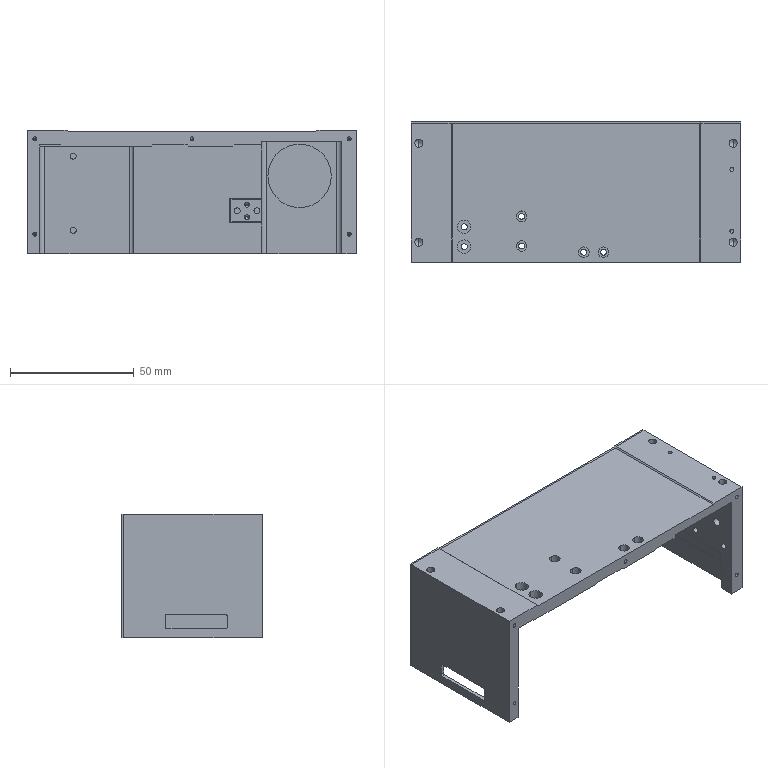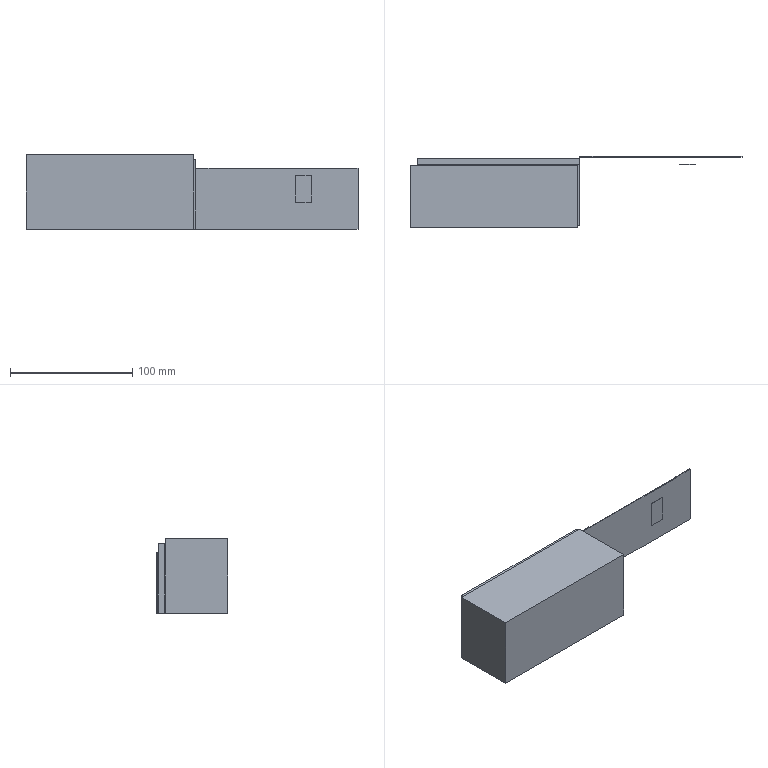CAM job | NX | 3+2 milling, drilling | part box 133 x 56.74 x 50 mm | stock box 272 x 58.74 x 60.74 mm
Tools:
number,name,description,diameter,corner_radius,flute_length,length,flutes
9,D10JING,Milling Tool-5 Parameters,10.0,0.0,50.0,75.0,2
10,D10,Milling Tool-5 Parameters,10.0,0.0,50.0,75.0,2
7,D6A45,Milling Tool-5 Parameters,6.0,0.0,50.0,75.0,2
13,3.3ZT,Drilling Tool,3.3,0.0,35.0,50.0,2
14,1.6ZT,Drilling Tool,1.6,0.0,35.0,50.0,2
12,2.4ZT,Drilling Tool,2.4,0.0,35.0,50.0,2
3,D3,Milling Tool-5 Parameters,3.0,0.0,50.0,75.0,2
5,D6R0.5,Milling Tool-5 Parameters,6.0,0.5,50.0,75.0,2
4,D4,Milling Tool-5 Parameters,4.0,0.0,50.0,75.0,2
1,D1,Milling Tool-5 Parameters,1.0,0.0,50.0,75.0,2
8,2.5ZT,Drilling Tool,2.5,0.0,35.0,50.0,2
2,3.4ZT,Drilling Tool,3.4,0.0,35.0,50.0,2
6,D6,Milling Tool-5 Parameters,6.0,0.0,50.0,75.0,2
1,D6.5XYD,Thread Mill,6.5,0.0,0.635,50.0,2
Operations:
program,operation,operation_type,tool,method,geometry_group,spindle_rpm,surface_speed,feed_per_tooth,feed_cut,feed_plunge,cut_length_mm,path_length_mm,cut_time_min,machine_time_min
1夹着做,FLOOR_WALL,VolumeBased25DMillingOperation,D10JING,METHOD,A,9500.0,298.0,0.0658,1250.0,100.0,1979.737,2033.737,1.584,1.589
1夹着做,ZLEVEL_PROFILE,ZLevelMilling,D10,METHOD,A,9500.0,298.0,0.1316,2500.0,1000.0,41221.216,41328.216,16.511,16.522
1夹着做,FLOOR_WALL_1,VolumeBased25DMillingOperation,D10,METHOD,A,9500.0,298.0,0.1316,2500.0,1000.0,1422.197,1476.997,0.5725,0.578
1夹着做,DRILLING,Operation,D6A45,METHOD,A,5000.0,94.0,0.025,250.0,0.0,48.0,420.512,0.192,0.2293
1夹着做,DRILLING_COPY,Operation,3.3ZT,METHOD,A,2000.0,20.0,0.0375,150.0,0.0,39.6,355.46,0.264,0.2956
1夹着做,DRILLING_COPY_COPY,Operation,1.6ZT,METHOD,A,2000.0,20.0,0.0375,150.0,0.0,25.04,138.26,0.1669,0.1783
1夹着做,DRILLING_COPY_COPY_COPY,Operation,2.4ZT,METHOD,A,2000.0,20.0,0.0375,150.0,0.0,67.326,289.278,0.4488,0.471
1夹着做,HOLE_MILLING,CylinderMilling,D3,METHOD,A,9500.0,89.0,0.0658,1250.0,100.0,550.401,1022.392,0.4403,0.4875
1夹着做,ZLEVEL_PROFILE_1,ZLevelMilling,D6R0.5,METHOD,A,9500.0,89.0,0.1316,2500.0,1000.0,1019.768,1241.961,0.4133,0.4356
1夹着做,FLOOR_WALL_COPY,VolumeBased25DMillingOperation,D10JING,METHOD,A,9500.0,298.0,0.0658,1250.0,100.0,1370.057,1425.057,1.096,1.101
1夹着做,PLANAR_MILL,PlanarMilling,D6A45,METHOD,A,9500.0,179.0,0.0658,1250.0,100.0,193.324,410.592,0.1547,0.1764
1夹着做,PLANAR_MILL_COPY_1,PlanarMilling,D6A45,METHOD,A,9500.0,179.0,0.0658,1250.0,100.0,50.126,494.214,0.0401,0.0845
1夹着做,PLANAR_MILL_COPY,PlanarMilling,D6A45,METHOD,A,9500.0,179.0,0.0658,1250.0,100.0,205.295,386.773,0.1642,0.1824
1夹着做,PLANAR_MILL_COPY_COPY,PlanarMilling,D6A45,METHOD,A,9500.0,179.0,0.0658,1250.0,100.0,97.215,533.447,0.0778,0.1214
1夹着做,刀补9,ZLevelMilling,D10JING,METHOD,A,9500.0,298.0,0.0632,1200.0,1000.0,1261.303,1636.159,1.053,1.091
2,ZLEVEL_PROFILE_COPY,ZLevelMilling,D4,METHOD,B,9500.0,119.0,0.1053,2000.0,1000.0,276.091,334.591,0.1552,0.1611
2,ZLEVEL_PROFILE_COPY_COPY,ZLevelMilling,D4,METHOD,B,9500.0,119.0,0.0526,1000.0,1000.0,53.319,108.819,0.0533,0.0589
2,ZLEVEL_PROFILE_COPY_COPY_1,ZLevelMilling,D1,METHOD,B,9500.0,29.0,0.0421,800.0,800.0,432.873,851.718,0.5411,0.583
2,PLANAR_MILL_COPY_1_COPY,PlanarMilling,D6A45,METHOD,B,9500.0,179.0,0.0658,1250.0,100.0,60.911,119.911,0.0487,0.0546
3,DRILLING_COPY_1,Operation,D6A45,METHOD,C,5000.0,94.0,0.025,250.0,0.0,40.0,265.781,0.16,0.1826
3,DRILLING_COPY_COPY_COPY_COPY,Operation,2.5ZT,METHOD,C,2000.0,20.0,0.0375,150.0,0.0,67.507,317.245,0.45,0.475
3,DRILLING_COPY_COPY_COPY_COPY_COPY,Operation,3.4ZT,METHOD,C,2000.0,20.0,0.0375,150.0,0.0,32.486,175.122,0.2166,0.2308
3,HOLE_MILLING_COPY,CylinderMilling,D4,METHOD,C,9500.0,89.0,0.0658,1250.0,100.0,752.275,1036.875,0.6018,0.6303
3,PLANAR_MILL_COPY_1_COPY_COPY,PlanarMilling,D6A45,METHOD,C,9500.0,179.0,0.0658,1250.0,100.0,158.952,844.34,0.1272,0.1957
4,FLOOR_WALL_COPY_1,VolumeBased25DMillingOperation,D10,METHOD,D,9500.0,298.0,0.0658,1250.0,100.0,12087.37,13055.906,9.67,9.767
4,FLOOR_WALL_COPY_2,VolumeBased25DMillingOperation,D10JING,METHOD,D,9500.0,298.0,0.0658,1250.0,100.0,1780.737,1834.737,1.425,1.43
4,DRILLING_COPY_1_COPY,Operation,D6A45,METHOD,D,5000.0,94.0,0.025,250.0,0.0,28.0,362.29,0.112,0.1454
4,DRILLING_COPY_COPY_COPY_1,Operation,1.6ZT,METHOD,D,2000.0,20.0,0.0375,150.0,0.0,92.04,490.371,0.6136,0.6534
4,CAVITY_MILL,CavityMilling,D10,METHOD,D,9500.0,298.0,0.1579,3000.0,1000.0,91249.531,91544.571,32.35,32.379
4,CAVITY_MILL_COPY,CavityMilling,D6,METHOD,D,9509.0,179.0,0.0789,1500.0,1000.0,5616.266,9526.694,4.418,4.809
4,11,ZLevelMilling,D10JING,METHOD,D,9500.0,298.0,0.0632,1200.0,1000.0,231.263,312.063,0.1935,0.2016
4,111,ZLevelMilling,D10JING,METHOD,D,9500.0,298.0,0.0632,1200.0,1000.0,1152.554,2284.3,0.9651,1.078
4,FLOOR_WALL_2,VolumeBased25DMillingOperation,D10JING,METHOD,D,9500.0,298.0,0.0658,1250.0,100.0,2218.259,4373.086,1.775,1.99
4,CAVITY_MILL_COPY_COPY,CavityMilling,D4,METHOD,D,7509.0,94.0,0.0666,1000.0,1000.0,9983.982,16148.265,9.984,10.6
4,PLANAR_PROFILE,PlanarMilling,D4,METHOD,D,6000.0,75.0,0.0667,800.0,100.0,702.0,1437.05,0.8775,0.951
4,ZLEVEL_PROFILE_1_COPY,ZLevelMilling,D6R0.5,METHOD,D,9500.0,89.0,0.1053,2000.0,1000.0,131.328,211.622,0.068,0.076
4,ZLEVEL_PROFILE_1_COPY_COPY,ZLevelMilling,D6R0.5,METHOD,D,9500.0,89.0,0.1053,2000.0,1000.0,829.791,1369.648,0.4217,0.4757
4,DRILLING_COPY_1_COPY_COPY,Operation,D6A45,METHOD,D,5000.0,94.0,0.025,250.0,0.0,28.0,296.013,0.112,0.1388
4,PLANAR_MILL_COPY_1_COPY_COPY_COPY,PlanarMilling,D6A45,METHOD,D,9500.0,179.0,0.0658,1250.0,100.0,507.377,566.377,0.4059,0.4118
5,DRILLING_COPY_1_COPY_COPY_1,Operation,D6A45,METHOD,E,5000.0,94.0,0.025,250.0,0.0,28.0,520.107,0.112,0.1612
5,DRILLING_COPY_COPY_COPY_1_COPY,Operation,1.6ZT,METHOD,E,2000.0,20.0,0.0375,150.0,0.0,41.0,421.84,0.2733,0.3114
5,PLANAR_MILL_1,PlanarMilling,D10JING,METHOD,E,8000.0,251.0,0.0781,1250.0,100.0,136.189,298.332,0.109,0.1252
6,FLOOR_WALL_1_COPY,VolumeBased25DMillingOperation,D10,METHOD,F,9500.0,298.0,0.1316,2500.0,1000.0,3857.286,3996.696,1.55,1.564
6,HOLE_MILLING_1,CylinderMilling,D10,METHOD,F,9500.0,298.0,0.0868,1650.0,100.0,454.605,522.085,0.2755,0.2823
6,FLOOR_WALL_COPY_COPY,VolumeBased25DMillingOperation,D10JING,METHOD,F,9500.0,298.0,0.0658,1250.0,100.0,1529.884,1874.592,1.224,1.258
6,11_COPY,ZLevelMilling,D10JING,METHOD,F,9500.0,298.0,0.0632,1200.0,1000.0,59.492,122.972,0.0504,0.0568
6,DRILLING_COPY_1_COPY_COPY_1_COPY,Operation,D6A45,METHOD,F,5000.0,94.0,0.025,250.0,0.0,16.0,207.956,0.064,0.0832
6,DRILLING_COPY_COPY_COPY_COPY_1,Operation,2.4ZT,METHOD,F,2000.0,20.0,0.0375,150.0,0.0,43.884,263.724,0.2926,0.3145
6,HOLE_MILLING_COPY_1,CylinderMilling,D3,METHOD,F,9500.0,89.0,0.0658,1250.0,100.0,337.757,696.992,0.2702,0.3061
6,PLANAR_MILL_COPY_1_COPY_COPY_COPY_COPY,PlanarMilling,D6A45,METHOD,F,9500.0,179.0,0.0658,1250.0,100.0,81.841,140.841,0.0655,0.0714
6,PLANAR_MILL_COPY_1_COPY_COPY_COPY_COPY_COPY,PlanarMilling,D6A45,METHOD,F,9500.0,179.0,0.0658,1250.0,100.0,435.791,909.301,0.3486,0.396
7,THREAD_MILLING,ThreadMilling,D6.5XYD,METHOD,F,5000.0,102.0,0.125,1250.0,100.0,2210.348,2290.426,1.768,1.776